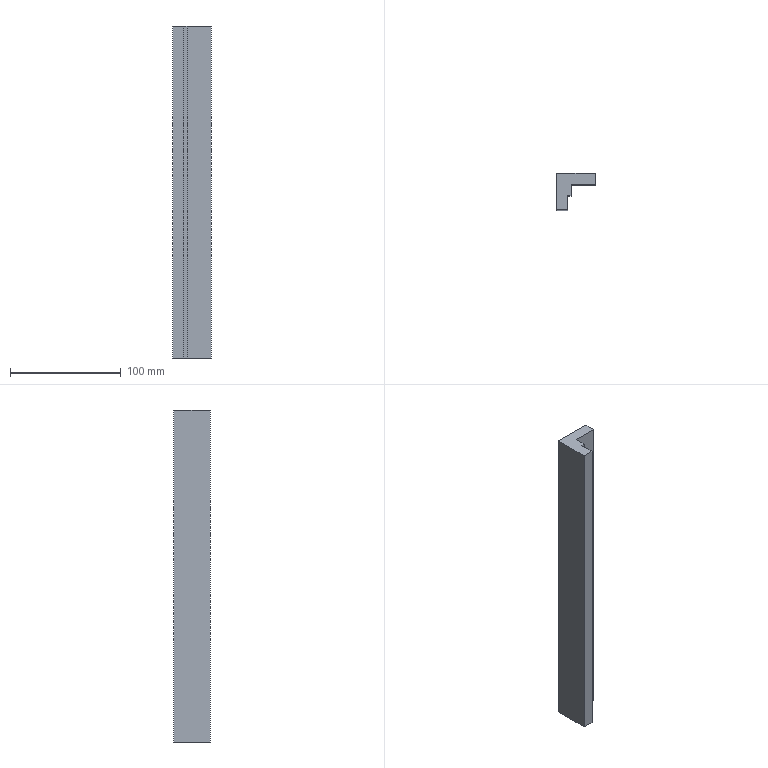Part | STEP file | Platform 2 slider plate 1 | 1 solid | 10 faces | box 35 x 33 x 300 mm | volume 183000 mm3 | plane 10
STEP:
#1=CARTESIAN_POINT('',(35.,0.,-150.));
#2=VERTEX_POINT('',#1);
#3=CARTESIAN_POINT('',(0.,0.,-150.));
#4=VERTEX_POINT('',#3);
#5=CARTESIAN_POINT('',(0.,0.,-150.));
#6=DIRECTION('',(-1.,0.,0.));
#7=VECTOR('',#6,1000.);
#8=LINE('',#5,#7);
#9=EDGE_CURVE('',#2,#4,#8,.T.);
#10=ORIENTED_EDGE('',*,*,#9,.T.);
#11=CARTESIAN_POINT('',(0.,0.,150.));
#12=VERTEX_POINT('',#11);
#13=CARTESIAN_POINT('',(0.,0.,150.));
#14=DIRECTION('',(0.,0.,-1.));
#15=VECTOR('',#14,1000.);
#16=LINE('',#13,#15);
#17=EDGE_CURVE('',#12,#4,#16,.T.);
#18=ORIENTED_EDGE('',*,*,#17,.F.);
#19=CARTESIAN_POINT('',(35.,0.,150.));
#20=VERTEX_POINT('',#19);
#21=CARTESIAN_POINT('',(0.,0.,150.));
#22=DIRECTION('',(-1.,0.,0.));
#23=VECTOR('',#22,1000.);
#24=LINE('',#21,#23);
#25=EDGE_CURVE('',#20,#12,#24,.T.);
#26=ORIENTED_EDGE('',*,*,#25,.F.);
#27=CARTESIAN_POINT('',(35.,0.,150.));
#28=DIRECTION('',(0.,0.,-1.));
#29=VECTOR('',#28,1000.);
#30=LINE('',#27,#29);
#31=EDGE_CURVE('',#20,#2,#30,.T.);
#32=ORIENTED_EDGE('',*,*,#31,.T.);
#33=EDGE_LOOP('',(#10,#18,#26,#32));
#34=FACE_OUTER_BOUND('',#33,.T.);
#35=CARTESIAN_POINT('',(0.,0.,150.));
#36=DIRECTION('',(0.,-1.,0.));
#37=DIRECTION('',(0.,0.,-1.));
#38=AXIS2_PLACEMENT_3D('',#35,#36,#37);
#39=PLANE('',#38);
#40=ADVANCED_FACE('',(#34),#39,.F.);
#41=CARTESIAN_POINT('',(0.,-33.,-150.));
#42=VERTEX_POINT('',#41);
#43=CARTESIAN_POINT('',(0.,0.,-150.));
#44=DIRECTION('',(0.,-1.,0.));
#45=VECTOR('',#44,1000.);
#46=LINE('',#43,#45);
#47=EDGE_CURVE('',#4,#42,#46,.T.);
#48=ORIENTED_EDGE('',*,*,#47,.T.);
#49=CARTESIAN_POINT('',(0.,-33.,150.));
#50=VERTEX_POINT('',#49);
#51=CARTESIAN_POINT('',(0.,-33.,150.));
#52=DIRECTION('',(0.,0.,-1.));
#53=VECTOR('',#52,1000.);
#54=LINE('',#51,#53);
#55=EDGE_CURVE('',#50,#42,#54,.T.);
#56=ORIENTED_EDGE('',*,*,#55,.F.);
#57=CARTESIAN_POINT('',(0.,0.,150.));
#58=DIRECTION('',(0.,-1.,0.));
#59=VECTOR('',#58,1000.);
#60=LINE('',#57,#59);
#61=EDGE_CURVE('',#12,#50,#60,.T.);
#62=ORIENTED_EDGE('',*,*,#61,.F.);
#63=ORIENTED_EDGE('',*,*,#17,.T.);
#64=EDGE_LOOP('',(#48,#56,#62,#63));
#65=FACE_OUTER_BOUND('',#64,.T.);
#66=CARTESIAN_POINT('',(0.,0.,150.));
#67=DIRECTION('',(1.,0.,0.));
#68=DIRECTION('',(0.,1.,0.));
#69=AXIS2_PLACEMENT_3D('',#66,#67,#68);
#70=PLANE('',#69);
#71=ADVANCED_FACE('',(#65),#70,.F.);
#72=CARTESIAN_POINT('',(10.,-33.,-150.));
#73=VERTEX_POINT('',#72);
#74=CARTESIAN_POINT('',(13.,-33.,-150.));
#75=DIRECTION('',(1.,0.,0.));
#76=VECTOR('',#75,1000.);
#77=LINE('',#74,#76);
#78=EDGE_CURVE('',#42,#73,#77,.T.);
#79=ORIENTED_EDGE('',*,*,#78,.T.);
#80=CARTESIAN_POINT('',(10.,-33.,150.));
#81=VERTEX_POINT('',#80);
#82=CARTESIAN_POINT('',(10.,-33.,-150.));
#83=DIRECTION('',(0.,0.,1.));
#84=VECTOR('',#83,1000.);
#85=LINE('',#82,#84);
#86=EDGE_CURVE('',#73,#81,#85,.T.);
#87=ORIENTED_EDGE('',*,*,#86,.T.);
#88=CARTESIAN_POINT('',(13.,-33.,150.));
#89=DIRECTION('',(1.,0.,0.));
#90=VECTOR('',#89,1000.);
#91=LINE('',#88,#90);
#92=EDGE_CURVE('',#50,#81,#91,.T.);
#93=ORIENTED_EDGE('',*,*,#92,.F.);
#94=ORIENTED_EDGE('',*,*,#55,.T.);
#95=EDGE_LOOP('',(#79,#87,#93,#94));
#96=FACE_OUTER_BOUND('',#95,.T.);
#97=CARTESIAN_POINT('',(13.,-33.,150.));
#98=DIRECTION('',(0.,1.,0.));
#99=DIRECTION('',(0.,0.,1.));
#100=AXIS2_PLACEMENT_3D('',#97,#98,#99);
#101=PLANE('',#100);
#102=ADVANCED_FACE('',(#96),#101,.F.);
#103=CARTESIAN_POINT('',(13.,-20.,150.));
#104=VERTEX_POINT('',#103);
#105=CARTESIAN_POINT('',(13.,-10.,150.));
#106=VERTEX_POINT('',#105);
#107=CARTESIAN_POINT('',(13.,-10.,150.));
#108=DIRECTION('',(0.,1.,0.));
#109=VECTOR('',#108,1000.);
#110=LINE('',#107,#109);
#111=EDGE_CURVE('',#104,#106,#110,.T.);
#112=ORIENTED_EDGE('',*,*,#111,.F.);
#113=CARTESIAN_POINT('',(13.,-20.,-150.));
#114=VERTEX_POINT('',#113);
#115=CARTESIAN_POINT('',(13.,-20.,-150.));
#116=DIRECTION('',(0.,0.,1.));
#117=VECTOR('',#116,1000.);
#118=LINE('',#115,#117);
#119=EDGE_CURVE('',#114,#104,#118,.T.);
#120=ORIENTED_EDGE('',*,*,#119,.F.);
#121=CARTESIAN_POINT('',(13.,-10.,-150.));
#122=VERTEX_POINT('',#121);
#123=CARTESIAN_POINT('',(13.,-10.,-150.));
#124=DIRECTION('',(0.,1.,0.));
#125=VECTOR('',#124,1000.);
#126=LINE('',#123,#125);
#127=EDGE_CURVE('',#114,#122,#126,.T.);
#128=ORIENTED_EDGE('',*,*,#127,.T.);
#129=CARTESIAN_POINT('',(13.,-10.,150.));
#130=DIRECTION('',(0.,0.,-1.));
#131=VECTOR('',#130,1000.);
#132=LINE('',#129,#131);
#133=EDGE_CURVE('',#106,#122,#132,.T.);
#134=ORIENTED_EDGE('',*,*,#133,.F.);
#135=EDGE_LOOP('',(#112,#120,#128,#134));
#136=FACE_OUTER_BOUND('',#135,.T.);
#137=CARTESIAN_POINT('',(13.,-10.,150.));
#138=DIRECTION('',(-1.,0.,0.));
#139=DIRECTION('',(0.,-1.,0.));
#140=AXIS2_PLACEMENT_3D('',#137,#138,#139);
#141=PLANE('',#140);
#142=ADVANCED_FACE('',(#136),#141,.F.);
#143=CARTESIAN_POINT('',(35.,-10.,-150.));
#144=VERTEX_POINT('',#143);
#145=CARTESIAN_POINT('',(35.,-10.,-150.));
#146=DIRECTION('',(1.,0.,0.));
#147=VECTOR('',#146,1000.);
#148=LINE('',#145,#147);
#149=EDGE_CURVE('',#122,#144,#148,.T.);
#150=ORIENTED_EDGE('',*,*,#149,.T.);
#151=CARTESIAN_POINT('',(35.,-10.,150.));
#152=VERTEX_POINT('',#151);
#153=CARTESIAN_POINT('',(35.,-10.,150.));
#154=DIRECTION('',(0.,0.,-1.));
#155=VECTOR('',#154,1000.);
#156=LINE('',#153,#155);
#157=EDGE_CURVE('',#152,#144,#156,.T.);
#158=ORIENTED_EDGE('',*,*,#157,.F.);
#159=CARTESIAN_POINT('',(35.,-10.,150.));
#160=DIRECTION('',(1.,0.,0.));
#161=VECTOR('',#160,1000.);
#162=LINE('',#159,#161);
#163=EDGE_CURVE('',#106,#152,#162,.T.);
#164=ORIENTED_EDGE('',*,*,#163,.F.);
#165=ORIENTED_EDGE('',*,*,#133,.T.);
#166=EDGE_LOOP('',(#150,#158,#164,#165));
#167=FACE_OUTER_BOUND('',#166,.T.);
#168=CARTESIAN_POINT('',(35.,-10.,150.));
#169=DIRECTION('',(0.,1.,0.));
#170=DIRECTION('',(-1.,0.,0.));
#171=AXIS2_PLACEMENT_3D('',#168,#169,#170);
#172=PLANE('',#171);
#173=ADVANCED_FACE('',(#167),#172,.F.);
#174=CARTESIAN_POINT('',(35.,0.,-150.));
#175=DIRECTION('',(0.,1.,0.));
#176=VECTOR('',#175,1000.);
#177=LINE('',#174,#176);
#178=EDGE_CURVE('',#144,#2,#177,.T.);
#179=ORIENTED_EDGE('',*,*,#178,.T.);
#180=ORIENTED_EDGE('',*,*,#31,.F.);
#181=CARTESIAN_POINT('',(35.,0.,150.));
#182=DIRECTION('',(0.,1.,0.));
#183=VECTOR('',#182,1000.);
#184=LINE('',#181,#183);
#185=EDGE_CURVE('',#152,#20,#184,.T.);
#186=ORIENTED_EDGE('',*,*,#185,.F.);
#187=ORIENTED_EDGE('',*,*,#157,.T.);
#188=EDGE_LOOP('',(#179,#180,#186,#187));
#189=FACE_OUTER_BOUND('',#188,.T.);
#190=CARTESIAN_POINT('',(35.,0.,150.));
#191=DIRECTION('',(-1.,0.,0.));
#192=DIRECTION('',(0.,0.,1.));
#193=AXIS2_PLACEMENT_3D('',#190,#191,#192);
#194=PLANE('',#193);
#195=ADVANCED_FACE('',(#189),#194,.F.);
#196=ORIENTED_EDGE('',*,*,#92,.T.);
#197=CARTESIAN_POINT('',(10.,-20.,150.));
#198=VERTEX_POINT('',#197);
#199=CARTESIAN_POINT('',(10.,-33.,150.));
#200=DIRECTION('',(0.,-1.,0.));
#201=VECTOR('',#200,1000.);
#202=LINE('',#199,#201);
#203=EDGE_CURVE('',#198,#81,#202,.T.);
#204=ORIENTED_EDGE('',*,*,#203,.F.);
#205=CARTESIAN_POINT('',(13.,-20.,150.));
#206=DIRECTION('',(-1.,0.,0.));
#207=VECTOR('',#206,1000.);
#208=LINE('',#205,#207);
#209=EDGE_CURVE('',#104,#198,#208,.T.);
#210=ORIENTED_EDGE('',*,*,#209,.F.);
#211=ORIENTED_EDGE('',*,*,#111,.T.);
#212=ORIENTED_EDGE('',*,*,#163,.T.);
#213=ORIENTED_EDGE('',*,*,#185,.T.);
#214=ORIENTED_EDGE('',*,*,#25,.T.);
#215=ORIENTED_EDGE('',*,*,#61,.T.);
#216=EDGE_LOOP('',(#196,#204,#210,#211,#212,#213,#214,#215));
#217=FACE_OUTER_BOUND('',#216,.T.);
#218=CARTESIAN_POINT('',(0.,0.,150.));
#219=DIRECTION('',(0.,0.,-1.));
#220=DIRECTION('',(-1.,0.,0.));
#221=AXIS2_PLACEMENT_3D('',#218,#219,#220);
#222=PLANE('',#221);
#223=ADVANCED_FACE('',(#217),#222,.F.);
#224=CARTESIAN_POINT('',(10.,-20.,-150.));
#225=VERTEX_POINT('',#224);
#226=CARTESIAN_POINT('',(10.,-33.,-150.));
#227=DIRECTION('',(0.,-1.,0.));
#228=VECTOR('',#227,1000.);
#229=LINE('',#226,#228);
#230=EDGE_CURVE('',#225,#73,#229,.T.);
#231=ORIENTED_EDGE('',*,*,#230,.T.);
#232=ORIENTED_EDGE('',*,*,#78,.F.);
#233=ORIENTED_EDGE('',*,*,#47,.F.);
#234=ORIENTED_EDGE('',*,*,#9,.F.);
#235=ORIENTED_EDGE('',*,*,#178,.F.);
#236=ORIENTED_EDGE('',*,*,#149,.F.);
#237=ORIENTED_EDGE('',*,*,#127,.F.);
#238=CARTESIAN_POINT('',(13.,-20.,-150.));
#239=DIRECTION('',(-1.,0.,0.));
#240=VECTOR('',#239,1000.);
#241=LINE('',#238,#240);
#242=EDGE_CURVE('',#114,#225,#241,.T.);
#243=ORIENTED_EDGE('',*,*,#242,.T.);
#244=EDGE_LOOP('',(#231,#232,#233,#234,#235,#236,#237,#243));
#245=FACE_OUTER_BOUND('',#244,.T.);
#246=CARTESIAN_POINT('',(0.,0.,-150.));
#247=DIRECTION('',(0.,0.,-1.));
#248=DIRECTION('',(-1.,0.,0.));
#249=AXIS2_PLACEMENT_3D('',#246,#247,#248);
#250=PLANE('',#249);
#251=ADVANCED_FACE('',(#245),#250,.T.);
#252=ORIENTED_EDGE('',*,*,#203,.T.);
#253=ORIENTED_EDGE('',*,*,#86,.F.);
#254=ORIENTED_EDGE('',*,*,#230,.F.);
#255=CARTESIAN_POINT('',(10.,-20.,-150.));
#256=DIRECTION('',(0.,0.,1.));
#257=VECTOR('',#256,1000.);
#258=LINE('',#255,#257);
#259=EDGE_CURVE('',#225,#198,#258,.T.);
#260=ORIENTED_EDGE('',*,*,#259,.T.);
#261=EDGE_LOOP('',(#252,#253,#254,#260));
#262=FACE_OUTER_BOUND('',#261,.T.);
#263=CARTESIAN_POINT('',(10.,-33.,-150.));
#264=DIRECTION('',(-1.,0.,0.));
#265=DIRECTION('',(0.,0.,1.));
#266=AXIS2_PLACEMENT_3D('',#263,#264,#265);
#267=PLANE('',#266);
#268=ADVANCED_FACE('',(#262),#267,.F.);
#269=ORIENTED_EDGE('',*,*,#209,.T.);
#270=ORIENTED_EDGE('',*,*,#259,.F.);
#271=ORIENTED_EDGE('',*,*,#242,.F.);
#272=ORIENTED_EDGE('',*,*,#119,.T.);
#273=EDGE_LOOP('',(#269,#270,#271,#272));
#274=FACE_OUTER_BOUND('',#273,.T.);
#275=CARTESIAN_POINT('',(13.,-20.,-150.));
#276=DIRECTION('',(0.,1.,0.));
#277=DIRECTION('',(0.,0.,1.));
#278=AXIS2_PLACEMENT_3D('',#275,#276,#277);
#279=PLANE('',#278);
#280=ADVANCED_FACE('',(#274),#279,.F.);
#281=CLOSED_SHELL('',(#40,#71,#102,#142,#173,#195,#223,#251,#268,#280));
#282=MANIFOLD_SOLID_BREP('',#281);
#283=CARTESIAN_POINT('',(0.,0.,0.));
#284=DIRECTION('',(0.,0.,1.));
#285=DIRECTION('',(1.,0.,0.));
#286=AXIS2_PLACEMENT_3D('',#283,#284,#285);
#287=(LENGTH_UNIT()NAMED_UNIT(*)SI_UNIT(.MILLI.,.METRE.));
#288=UNCERTAINTY_MEASURE_WITH_UNIT(LENGTH_MEASURE(0.00001),#287,'','');
#289=(NAMED_UNIT(*)PLANE_ANGLE_UNIT()SI_UNIT($,.RADIAN.));
#290=(NAMED_UNIT(*)SI_UNIT($,.STERADIAN.)SOLID_ANGLE_UNIT());
#291=(GEOMETRIC_REPRESENTATION_CONTEXT(3)GLOBAL_UNCERTAINTY_ASSIGNED_CONTEXT((#288))GLOBAL_UNIT_ASSIGNED_CONTEXT((#287,#289,#290))REPRESENTATION_CONTEXT('',''));
#292=ADVANCED_BREP_SHAPE_REPRESENTATION('',(#282,#286),#291);